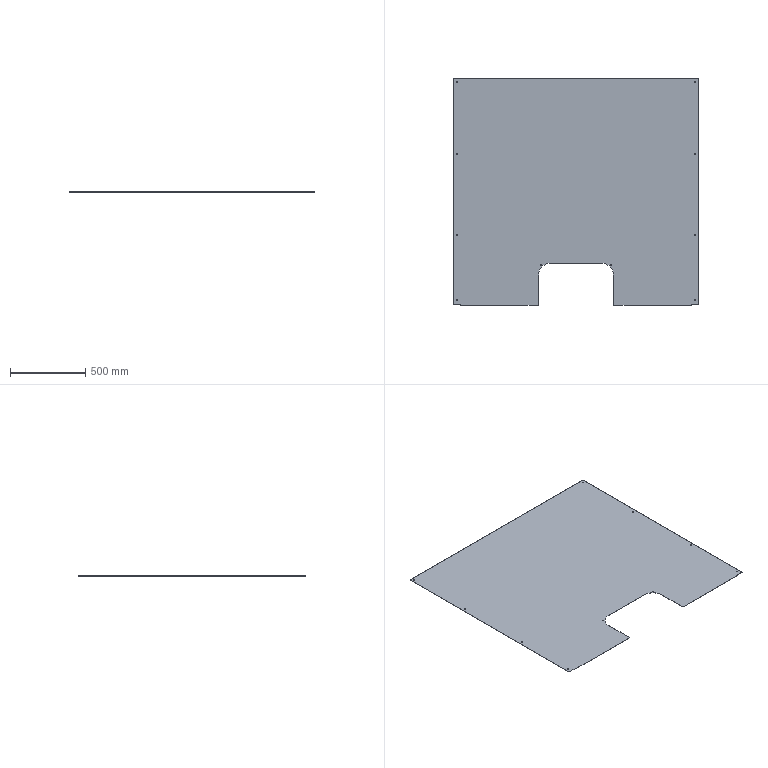Part | SolidWorks | features ICE 6, Fillet 3, HoleWzd 3, FlatPattern 1, SMBaseFlange 1, SheetMetal 1 | 1 solid | 44 faces | box 1628 x 1507 x 1.2 mm | volume 2778351 mm3 | cylinder 30 | plane 14 | commonest cylinder face diameters 7 x20 6 x8 160 x2
STEP:
#1=CARTESIAN_POINT('',(1511.5,-1240.,0.));
#2=VERTEX_POINT('',#1);
#3=CARTESIAN_POINT('',(1518.5,-1240.,0.));
#4=VERTEX_POINT('',#3);
#5=CARTESIAN_POINT('',(1515.,-1240.,0.));
#6=DIRECTION('',(0.,0.,1.));
#7=DIRECTION('',(1.,0.,0.));
#8=AXIS2_PLACEMENT_3D('',#5,#6,#7);
#9=CIRCLE('',#8,3.5);
#10=EDGE_CURVE('',#2,#4,#9,.T.);
#11=ORIENTED_EDGE('',*,*,#10,.F.);
#12=CARTESIAN_POINT('',(1511.5,-1240.,1.2));
#13=VERTEX_POINT('',#12);
#14=CARTESIAN_POINT('',(1511.5,-1240.,1.2));
#15=DIRECTION('',(0.,0.,1.));
#16=VECTOR('',#15,1000.);
#17=LINE('',#14,#16);
#18=EDGE_CURVE('',#2,#13,#17,.T.);
#19=ORIENTED_EDGE('',*,*,#18,.T.);
#20=CARTESIAN_POINT('',(1518.5,-1240.,1.2));
#21=VERTEX_POINT('',#20);
#22=CARTESIAN_POINT('',(1515.,-1240.,1.2));
#23=DIRECTION('',(0.,0.,1.));
#24=DIRECTION('',(1.,0.,0.));
#25=AXIS2_PLACEMENT_3D('',#22,#23,#24);
#26=CIRCLE('',#25,3.5);
#27=EDGE_CURVE('',#13,#21,#26,.T.);
#28=ORIENTED_EDGE('',*,*,#27,.T.);
#29=CARTESIAN_POINT('',(1518.5,-1240.,1.2));
#30=DIRECTION('',(0.,0.,1.));
#31=VECTOR('',#30,1000.);
#32=LINE('',#29,#31);
#33=EDGE_CURVE('',#4,#21,#32,.T.);
#34=ORIENTED_EDGE('',*,*,#33,.F.);
#35=EDGE_LOOP('',(#11,#19,#28,#34));
#36=FACE_OUTER_BOUND('',#35,.T.);
#37=CARTESIAN_POINT('',(1515.,-1240.,1.2));
#38=DIRECTION('',(0.,0.,1.));
#39=DIRECTION('',(1.,0.,0.));
#40=AXIS2_PLACEMENT_3D('',#37,#38,#39);
#41=CYLINDRICAL_SURFACE('',#40,3.5);
#42=ADVANCED_FACE('',(#36),#41,.F.);
#43=CARTESIAN_POINT('',(1981.5,-1240.,0.));
#44=VERTEX_POINT('',#43);
#45=CARTESIAN_POINT('',(1988.5,-1240.,0.));
#46=VERTEX_POINT('',#45);
#47=CARTESIAN_POINT('',(1985.,-1240.,0.));
#48=DIRECTION('',(0.,0.,1.));
#49=DIRECTION('',(1.,0.,0.));
#50=AXIS2_PLACEMENT_3D('',#47,#48,#49);
#51=CIRCLE('',#50,3.5);
#52=EDGE_CURVE('',#44,#46,#51,.T.);
#53=ORIENTED_EDGE('',*,*,#52,.F.);
#54=CARTESIAN_POINT('',(1981.5,-1240.,1.2));
#55=VERTEX_POINT('',#54);
#56=CARTESIAN_POINT('',(1981.5,-1240.,1.2));
#57=DIRECTION('',(0.,0.,1.));
#58=VECTOR('',#57,1000.);
#59=LINE('',#56,#58);
#60=EDGE_CURVE('',#44,#55,#59,.T.);
#61=ORIENTED_EDGE('',*,*,#60,.T.);
#62=CARTESIAN_POINT('',(1988.5,-1240.,1.2));
#63=VERTEX_POINT('',#62);
#64=CARTESIAN_POINT('',(1985.,-1240.,1.2));
#65=DIRECTION('',(0.,0.,1.));
#66=DIRECTION('',(1.,0.,0.));
#67=AXIS2_PLACEMENT_3D('',#64,#65,#66);
#68=CIRCLE('',#67,3.5);
#69=EDGE_CURVE('',#55,#63,#68,.T.);
#70=ORIENTED_EDGE('',*,*,#69,.T.);
#71=CARTESIAN_POINT('',(1988.5,-1240.,1.2));
#72=DIRECTION('',(0.,0.,1.));
#73=VECTOR('',#72,1000.);
#74=LINE('',#71,#73);
#75=EDGE_CURVE('',#46,#63,#74,.T.);
#76=ORIENTED_EDGE('',*,*,#75,.F.);
#77=EDGE_LOOP('',(#53,#61,#70,#76));
#78=FACE_OUTER_BOUND('',#77,.T.);
#79=CARTESIAN_POINT('',(1985.,-1240.,1.2));
#80=DIRECTION('',(0.,0.,1.));
#81=DIRECTION('',(1.,0.,0.));
#82=AXIS2_PLACEMENT_3D('',#79,#80,#81);
#83=CYLINDRICAL_SURFACE('',#82,3.5);
#84=ADVANCED_FACE('',(#78),#83,.F.);
#85=CARTESIAN_POINT('',(952.5,-20.,0.));
#86=VERTEX_POINT('',#85);
#87=CARTESIAN_POINT('',(959.5,-20.,0.));
#88=VERTEX_POINT('',#87);
#89=CARTESIAN_POINT('',(956.,-20.,0.));
#90=DIRECTION('',(0.,0.,1.));
#91=DIRECTION('',(1.,0.,0.));
#92=AXIS2_PLACEMENT_3D('',#89,#90,#91);
#93=CIRCLE('',#92,3.5);
#94=EDGE_CURVE('',#86,#88,#93,.T.);
#95=ORIENTED_EDGE('',*,*,#94,.F.);
#96=CARTESIAN_POINT('',(952.5,-20.,1.2));
#97=VERTEX_POINT('',#96);
#98=CARTESIAN_POINT('',(952.5,-20.,1.2));
#99=DIRECTION('',(0.,0.,1.));
#100=VECTOR('',#99,1000.);
#101=LINE('',#98,#100);
#102=EDGE_CURVE('',#86,#97,#101,.T.);
#103=ORIENTED_EDGE('',*,*,#102,.T.);
#104=CARTESIAN_POINT('',(959.5,-20.,1.2));
#105=VERTEX_POINT('',#104);
#106=CARTESIAN_POINT('',(956.,-20.,1.2));
#107=DIRECTION('',(0.,0.,1.));
#108=DIRECTION('',(1.,0.,0.));
#109=AXIS2_PLACEMENT_3D('',#106,#107,#108);
#110=CIRCLE('',#109,3.5);
#111=EDGE_CURVE('',#97,#105,#110,.T.);
#112=ORIENTED_EDGE('',*,*,#111,.T.);
#113=CARTESIAN_POINT('',(959.5,-20.,1.2));
#114=DIRECTION('',(0.,0.,1.));
#115=VECTOR('',#114,1000.);
#116=LINE('',#113,#115);
#117=EDGE_CURVE('',#88,#105,#116,.T.);
#118=ORIENTED_EDGE('',*,*,#117,.F.);
#119=EDGE_LOOP('',(#95,#103,#112,#118));
#120=FACE_OUTER_BOUND('',#119,.T.);
#121=CARTESIAN_POINT('',(956.,-20.,1.2));
#122=DIRECTION('',(0.,0.,1.));
#123=DIRECTION('',(1.,0.,0.));
#124=AXIS2_PLACEMENT_3D('',#121,#122,#123);
#125=CYLINDRICAL_SURFACE('',#124,3.5);
#126=ADVANCED_FACE('',(#120),#125,.F.);
#127=CARTESIAN_POINT('',(2540.5,-20.,0.));
#128=VERTEX_POINT('',#127);
#129=CARTESIAN_POINT('',(2547.5,-20.,0.));
#130=VERTEX_POINT('',#129);
#131=CARTESIAN_POINT('',(2544.,-20.,0.));
#132=DIRECTION('',(0.,0.,1.));
#133=DIRECTION('',(1.,0.,0.));
#134=AXIS2_PLACEMENT_3D('',#131,#132,#133);
#135=CIRCLE('',#134,3.5);
#136=EDGE_CURVE('',#128,#130,#135,.T.);
#137=ORIENTED_EDGE('',*,*,#136,.F.);
#138=CARTESIAN_POINT('',(2540.5,-20.,1.2));
#139=VERTEX_POINT('',#138);
#140=CARTESIAN_POINT('',(2540.5,-20.,1.2));
#141=DIRECTION('',(0.,0.,1.));
#142=VECTOR('',#141,1000.);
#143=LINE('',#140,#142);
#144=EDGE_CURVE('',#128,#139,#143,.T.);
#145=ORIENTED_EDGE('',*,*,#144,.T.);
#146=CARTESIAN_POINT('',(2547.5,-20.,1.2));
#147=VERTEX_POINT('',#146);
#148=CARTESIAN_POINT('',(2544.,-20.,1.2));
#149=DIRECTION('',(0.,0.,1.));
#150=DIRECTION('',(1.,0.,0.));
#151=AXIS2_PLACEMENT_3D('',#148,#149,#150);
#152=CIRCLE('',#151,3.5);
#153=EDGE_CURVE('',#139,#147,#152,.T.);
#154=ORIENTED_EDGE('',*,*,#153,.T.);
#155=CARTESIAN_POINT('',(2547.5,-20.,1.2));
#156=DIRECTION('',(0.,0.,1.));
#157=VECTOR('',#156,1000.);
#158=LINE('',#155,#157);
#159=EDGE_CURVE('',#130,#147,#158,.T.);
#160=ORIENTED_EDGE('',*,*,#159,.F.);
#161=EDGE_LOOP('',(#137,#145,#154,#160));
#162=FACE_OUTER_BOUND('',#161,.T.);
#163=CARTESIAN_POINT('',(2544.,-20.,1.2));
#164=DIRECTION('',(0.,0.,1.));
#165=DIRECTION('',(1.,0.,0.));
#166=AXIS2_PLACEMENT_3D('',#163,#164,#165);
#167=CYLINDRICAL_SURFACE('',#166,3.5);
#168=ADVANCED_FACE('',(#162),#167,.F.);
#169=CARTESIAN_POINT('',(952.5,-1471.,0.));
#170=VERTEX_POINT('',#169);
#171=CARTESIAN_POINT('',(959.5,-1471.,0.));
#172=VERTEX_POINT('',#171);
#173=CARTESIAN_POINT('',(956.,-1471.,0.));
#174=DIRECTION('',(0.,0.,1.));
#175=DIRECTION('',(1.,0.,0.));
#176=AXIS2_PLACEMENT_3D('',#173,#174,#175);
#177=CIRCLE('',#176,3.5);
#178=EDGE_CURVE('',#170,#172,#177,.T.);
#179=ORIENTED_EDGE('',*,*,#178,.F.);
#180=CARTESIAN_POINT('',(952.5,-1471.,1.2));
#181=VERTEX_POINT('',#180);
#182=CARTESIAN_POINT('',(952.5,-1471.,1.2));
#183=DIRECTION('',(0.,0.,1.));
#184=VECTOR('',#183,1000.);
#185=LINE('',#182,#184);
#186=EDGE_CURVE('',#170,#181,#185,.T.);
#187=ORIENTED_EDGE('',*,*,#186,.T.);
#188=CARTESIAN_POINT('',(959.5,-1471.,1.2));
#189=VERTEX_POINT('',#188);
#190=CARTESIAN_POINT('',(956.,-1471.,1.2));
#191=DIRECTION('',(0.,0.,1.));
#192=DIRECTION('',(1.,0.,0.));
#193=AXIS2_PLACEMENT_3D('',#190,#191,#192);
#194=CIRCLE('',#193,3.5);
#195=EDGE_CURVE('',#181,#189,#194,.T.);
#196=ORIENTED_EDGE('',*,*,#195,.T.);
#197=CARTESIAN_POINT('',(959.5,-1471.,1.2));
#198=DIRECTION('',(0.,0.,1.));
#199=VECTOR('',#198,1000.);
#200=LINE('',#197,#199);
#201=EDGE_CURVE('',#172,#189,#200,.T.);
#202=ORIENTED_EDGE('',*,*,#201,.F.);
#203=EDGE_LOOP('',(#179,#187,#196,#202));
#204=FACE_OUTER_BOUND('',#203,.T.);
#205=CARTESIAN_POINT('',(956.,-1471.,1.2));
#206=DIRECTION('',(0.,0.,1.));
#207=DIRECTION('',(1.,0.,0.));
#208=AXIS2_PLACEMENT_3D('',#205,#206,#207);
#209=CYLINDRICAL_SURFACE('',#208,3.5);
#210=ADVANCED_FACE('',(#204),#209,.F.);
#211=CARTESIAN_POINT('',(2540.5,-1471.,0.));
#212=VERTEX_POINT('',#211);
#213=CARTESIAN_POINT('',(2547.5,-1471.,0.));
#214=VERTEX_POINT('',#213);
#215=CARTESIAN_POINT('',(2544.,-1471.,0.));
#216=DIRECTION('',(0.,0.,1.));
#217=DIRECTION('',(1.,0.,0.));
#218=AXIS2_PLACEMENT_3D('',#215,#216,#217);
#219=CIRCLE('',#218,3.5);
#220=EDGE_CURVE('',#212,#214,#219,.T.);
#221=ORIENTED_EDGE('',*,*,#220,.F.);
#222=CARTESIAN_POINT('',(2540.5,-1471.,1.2));
#223=VERTEX_POINT('',#222);
#224=CARTESIAN_POINT('',(2540.5,-1471.,1.2));
#225=DIRECTION('',(0.,0.,1.));
#226=VECTOR('',#225,1000.);
#227=LINE('',#224,#226);
#228=EDGE_CURVE('',#212,#223,#227,.T.);
#229=ORIENTED_EDGE('',*,*,#228,.T.);
#230=CARTESIAN_POINT('',(2547.5,-1471.,1.2));
#231=VERTEX_POINT('',#230);
#232=CARTESIAN_POINT('',(2544.,-1471.,1.2));
#233=DIRECTION('',(0.,0.,1.));
#234=DIRECTION('',(1.,0.,0.));
#235=AXIS2_PLACEMENT_3D('',#232,#233,#234);
#236=CIRCLE('',#235,3.5);
#237=EDGE_CURVE('',#223,#231,#236,.T.);
#238=ORIENTED_EDGE('',*,*,#237,.T.);
#239=CARTESIAN_POINT('',(2547.5,-1471.,1.2));
#240=DIRECTION('',(0.,0.,1.));
#241=VECTOR('',#240,1000.);
#242=LINE('',#239,#241);
#243=EDGE_CURVE('',#214,#231,#242,.T.);
#244=ORIENTED_EDGE('',*,*,#243,.F.);
#245=EDGE_LOOP('',(#221,#229,#238,#244));
#246=FACE_OUTER_BOUND('',#245,.T.);
#247=CARTESIAN_POINT('',(2544.,-1471.,1.2));
#248=DIRECTION('',(0.,0.,1.));
#249=DIRECTION('',(1.,0.,0.));
#250=AXIS2_PLACEMENT_3D('',#247,#248,#249);
#251=CYLINDRICAL_SURFACE('',#250,3.5);
#252=ADVANCED_FACE('',(#246),#251,.F.);
#253=CARTESIAN_POINT('',(952.5,-1038.,0.));
#254=VERTEX_POINT('',#253);
#255=CARTESIAN_POINT('',(959.5,-1038.,0.));
#256=VERTEX_POINT('',#255);
#257=CARTESIAN_POINT('',(956.,-1038.,0.));
#258=DIRECTION('',(0.,0.,1.));
#259=DIRECTION('',(1.,0.,0.));
#260=AXIS2_PLACEMENT_3D('',#257,#258,#259);
#261=CIRCLE('',#260,3.5);
#262=EDGE_CURVE('',#254,#256,#261,.T.);
#263=ORIENTED_EDGE('',*,*,#262,.F.);
#264=CARTESIAN_POINT('',(952.5,-1038.,1.2));
#265=VERTEX_POINT('',#264);
#266=CARTESIAN_POINT('',(952.5,-1038.,1.2));
#267=DIRECTION('',(0.,0.,1.));
#268=VECTOR('',#267,1000.);
#269=LINE('',#266,#268);
#270=EDGE_CURVE('',#254,#265,#269,.T.);
#271=ORIENTED_EDGE('',*,*,#270,.T.);
#272=CARTESIAN_POINT('',(959.5,-1038.,1.2));
#273=VERTEX_POINT('',#272);
#274=CARTESIAN_POINT('',(956.,-1038.,1.2));
#275=DIRECTION('',(0.,0.,1.));
#276=DIRECTION('',(1.,0.,0.));
#277=AXIS2_PLACEMENT_3D('',#274,#275,#276);
#278=CIRCLE('',#277,3.5);
#279=EDGE_CURVE('',#265,#273,#278,.T.);
#280=ORIENTED_EDGE('',*,*,#279,.T.);
#281=CARTESIAN_POINT('',(959.5,-1038.,1.2));
#282=DIRECTION('',(0.,0.,1.));
#283=VECTOR('',#282,1000.);
#284=LINE('',#281,#283);
#285=EDGE_CURVE('',#256,#273,#284,.T.);
#286=ORIENTED_EDGE('',*,*,#285,.F.);
#287=EDGE_LOOP('',(#263,#271,#280,#286));
#288=FACE_OUTER_BOUND('',#287,.T.);
#289=CARTESIAN_POINT('',(956.,-1038.,1.2));
#290=DIRECTION('',(0.,0.,1.));
#291=DIRECTION('',(1.,0.,0.));
#292=AXIS2_PLACEMENT_3D('',#289,#290,#291);
#293=CYLINDRICAL_SURFACE('',#292,3.5);
#294=ADVANCED_FACE('',(#288),#293,.F.);
#295=CARTESIAN_POINT('',(2540.5,-1038.,0.));
#296=VERTEX_POINT('',#295);
#297=CARTESIAN_POINT('',(2547.5,-1038.,0.));
#298=VERTEX_POINT('',#297);
#299=CARTESIAN_POINT('',(2544.,-1038.,0.));
#300=DIRECTION('',(0.,0.,1.));
#301=DIRECTION('',(1.,0.,0.));
#302=AXIS2_PLACEMENT_3D('',#299,#300,#301);
#303=CIRCLE('',#302,3.5);
#304=EDGE_CURVE('',#296,#298,#303,.T.);
#305=ORIENTED_EDGE('',*,*,#304,.F.);
#306=CARTESIAN_POINT('',(2540.5,-1038.,1.2));
#307=VERTEX_POINT('',#306);
#308=CARTESIAN_POINT('',(2540.5,-1038.,1.2));
#309=DIRECTION('',(0.,0.,1.));
#310=VECTOR('',#309,1000.);
#311=LINE('',#308,#310);
#312=EDGE_CURVE('',#296,#307,#311,.T.);
#313=ORIENTED_EDGE('',*,*,#312,.T.);
#314=CARTESIAN_POINT('',(2547.5,-1038.,1.2));
#315=VERTEX_POINT('',#314);
#316=CARTESIAN_POINT('',(2544.,-1038.,1.2));
#317=DIRECTION('',(0.,0.,1.));
#318=DIRECTION('',(1.,0.,0.));
#319=AXIS2_PLACEMENT_3D('',#316,#317,#318);
#320=CIRCLE('',#319,3.5);
#321=EDGE_CURVE('',#307,#315,#320,.T.);
#322=ORIENTED_EDGE('',*,*,#321,.T.);
#323=CARTESIAN_POINT('',(2547.5,-1038.,1.2));
#324=DIRECTION('',(0.,0.,1.));
#325=VECTOR('',#324,1000.);
#326=LINE('',#323,#325);
#327=EDGE_CURVE('',#298,#315,#326,.T.);
#328=ORIENTED_EDGE('',*,*,#327,.F.);
#329=EDGE_LOOP('',(#305,#313,#322,#328));
#330=FACE_OUTER_BOUND('',#329,.T.);
#331=CARTESIAN_POINT('',(2544.,-1038.,1.2));
#332=DIRECTION('',(0.,0.,1.));
#333=DIRECTION('',(1.,0.,0.));
#334=AXIS2_PLACEMENT_3D('',#331,#332,#333);
#335=CYLINDRICAL_SURFACE('',#334,3.5);
#336=ADVANCED_FACE('',(#330),#335,.F.);
#337=CARTESIAN_POINT('',(952.5,-498.,0.));
#338=VERTEX_POINT('',#337);
#339=CARTESIAN_POINT('',(959.5,-498.,0.));
#340=VERTEX_POINT('',#339);
#341=CARTESIAN_POINT('',(956.,-498.,0.));
#342=DIRECTION('',(0.,0.,1.));
#343=DIRECTION('',(1.,0.,0.));
#344=AXIS2_PLACEMENT_3D('',#341,#342,#343);
#345=CIRCLE('',#344,3.5);
#346=EDGE_CURVE('',#338,#340,#345,.T.);
#347=ORIENTED_EDGE('',*,*,#346,.F.);
#348=CARTESIAN_POINT('',(952.5,-498.,1.2));
#349=VERTEX_POINT('',#348);
#350=CARTESIAN_POINT('',(952.5,-498.,1.2));
#351=DIRECTION('',(0.,0.,1.));
#352=VECTOR('',#351,1000.);
#353=LINE('',#350,#352);
#354=EDGE_CURVE('',#338,#349,#353,.T.);
#355=ORIENTED_EDGE('',*,*,#354,.T.);
#356=CARTESIAN_POINT('',(959.5,-498.,1.2));
#357=VERTEX_POINT('',#356);
#358=CARTESIAN_POINT('',(956.,-498.,1.2));
#359=DIRECTION('',(0.,0.,1.));
#360=DIRECTION('',(1.,0.,0.));
#361=AXIS2_PLACEMENT_3D('',#358,#359,#360);
#362=CIRCLE('',#361,3.5);
#363=EDGE_CURVE('',#349,#357,#362,.T.);
#364=ORIENTED_EDGE('',*,*,#363,.T.);
#365=CARTESIAN_POINT('',(959.5,-498.,1.2));
#366=DIRECTION('',(0.,0.,1.));
#367=VECTOR('',#366,1000.);
#368=LINE('',#365,#367);
#369=EDGE_CURVE('',#340,#357,#368,.T.);
#370=ORIENTED_EDGE('',*,*,#369,.F.);
#371=EDGE_LOOP('',(#347,#355,#364,#370));
#372=FACE_OUTER_BOUND('',#371,.T.);
#373=CARTESIAN_POINT('',(956.,-498.,1.2));
#374=DIRECTION('',(0.,0.,1.));
#375=DIRECTION('',(1.,0.,0.));
#376=AXIS2_PLACEMENT_3D('',#373,#374,#375);
#377=CYLINDRICAL_SURFACE('',#376,3.5);
#378=ADVANCED_FACE('',(#372),#377,.F.);
#379=CARTESIAN_POINT('',(2540.5,-498.,0.));
#380=VERTEX_POINT('',#379);
#381=CARTESIAN_POINT('',(2547.5,-498.,0.));
#382=VERTEX_POINT('',#381);
#383=CARTESIAN_POINT('',(2544.,-498.,0.));
#384=DIRECTION('',(0.,0.,1.));
#385=DIRECTION('',(1.,0.,0.));
#386=AXIS2_PLACEMENT_3D('',#383,#384,#385);
#387=CIRCLE('',#386,3.5);
#388=EDGE_CURVE('',#380,#382,#387,.T.);
#389=ORIENTED_EDGE('',*,*,#388,.F.);
#390=CARTESIAN_POINT('',(2540.5,-498.,1.2));
#391=VERTEX_POINT('',#390);
#392=CARTESIAN_POINT('',(2540.5,-498.,1.2));
#393=DIRECTION('',(0.,0.,1.));
#394=VECTOR('',#393,1000.);
#395=LINE('',#392,#394);
#396=EDGE_CURVE('',#380,#391,#395,.T.);
#397=ORIENTED_EDGE('',*,*,#396,.T.);
#398=CARTESIAN_POINT('',(2547.5,-498.,1.2));
#399=VERTEX_POINT('',#398);
#400=CARTESIAN_POINT('',(2544.,-498.,1.2));
#401=DIRECTION('',(0.,0.,1.));
#402=DIRECTION('',(1.,0.,0.));
#403=AXIS2_PLACEMENT_3D('',#400,#401,#402);
#404=CIRCLE('',#403,3.5);
#405=EDGE_CURVE('',#391,#399,#404,.T.);
#406=ORIENTED_EDGE('',*,*,#405,.T.);
#407=CARTESIAN_POINT('',(2547.5,-498.,1.2));
#408=DIRECTION('',(0.,0.,1.));
#409=VECTOR('',#408,1000.);
#410=LINE('',#407,#409);
#411=EDGE_CURVE('',#382,#399,#410,.T.);
#412=ORIENTED_EDGE('',*,*,#411,.F.);
#413=EDGE_LOOP('',(#389,#397,#406,#412));
#414=FACE_OUTER_BOUND('',#413,.T.);
#415=CARTESIAN_POINT('',(2544.,-498.,1.2));
#416=DIRECTION('',(0.,0.,1.));
#417=DIRECTION('',(1.,0.,0.));
#418=AXIS2_PLACEMENT_3D('',#415,#416,#417);
#419=CYLINDRICAL_SURFACE('',#418,3.5);
#420=ADVANCED_FACE('',(#414),#419,.F.);
#421=CARTESIAN_POINT('',(1497.,-1507.,1.2));
#422=VERTEX_POINT('',#421);
#423=CARTESIAN_POINT('',(984.,-1507.,1.2));
#424=VERTEX_POINT('',#423);
#425=CARTESIAN_POINT('',(890.,-1507.,1.2));
#426=DIRECTION('',(-1.,0.,0.));
#427=VECTOR('',#426,1000.);
#428=LINE('',#425,#427);
#429=EDGE_CURVE('',#422,#424,#428,.T.);
#430=ORIENTED_EDGE('',*,*,#429,.T.);
#431=CARTESIAN_POINT('',(984.,-1507.,0.));
#432=VERTEX_POINT('',#431);
#433=CARTESIAN_POINT('',(984.,-1507.,-8.8));
#434=DIRECTION('',(0.,0.,-1.));
#435=VECTOR('',#434,1000.);
#436=LINE('',#433,#435);
#437=EDGE_CURVE('',#424,#432,#436,.T.);
#438=ORIENTED_EDGE('',*,*,#437,.T.);
#439=CARTESIAN_POINT('',(1497.,-1507.,0.));
#440=VERTEX_POINT('',#439);
#441=CARTESIAN_POINT('',(0.,-1507.,0.));
#442=DIRECTION('',(-1.,0.,0.));
#443=VECTOR('',#442,1000.);
#444=LINE('',#441,#443);
#445=EDGE_CURVE('',#440,#432,#444,.T.);
#446=ORIENTED_EDGE('',*,*,#445,.F.);
#447=CARTESIAN_POINT('',(1497.,-1507.,-8.8));
#448=DIRECTION('',(0.,0.,1.));
#449=VECTOR('',#448,1000.);
#450=LINE('',#447,#449);
#451=EDGE_CURVE('',#440,#422,#450,.T.);
#452=ORIENTED_EDGE('',*,*,#451,.T.);
#453=EDGE_LOOP('',(#430,#438,#446,#452));
#454=FACE_OUTER_BOUND('',#453,.T.);
#455=CARTESIAN_POINT('',(890.,-1507.,-8.8));
#456=DIRECTION('',(0.,1.,0.));
#457=DIRECTION('',(0.,0.,1.));
#458=AXIS2_PLACEMENT_3D('',#455,#456,#457);
#459=PLANE('',#458);
#460=ADVANCED_FACE('',(#454),#459,.F.);
#461=CARTESIAN_POINT('',(939.,0.,0.));
#462=VERTEX_POINT('',#461);
#463=CARTESIAN_POINT('',(2561.,0.,0.));
#464=VERTEX_POINT('',#463);
#465=CARTESIAN_POINT('',(0.,0.,0.));
#466=DIRECTION('',(1.,0.,0.));
#467=VECTOR('',#466,1000.);
#468=LINE('',#465,#467);
#469=EDGE_CURVE('',#462,#464,#468,.T.);
#470=ORIENTED_EDGE('',*,*,#469,.F.);
#471=CARTESIAN_POINT('',(939.,0.,1.2));
#472=VERTEX_POINT('',#471);
#473=CARTESIAN_POINT('',(939.,0.,1.2));
#474=DIRECTION('',(0.,0.,1.));
#475=VECTOR('',#474,1000.);
#476=LINE('',#473,#475);
#477=EDGE_CURVE('',#462,#472,#476,.T.);
#478=ORIENTED_EDGE('',*,*,#477,.T.);
#479=CARTESIAN_POINT('',(2561.,0.,1.2));
#480=VERTEX_POINT('',#479);
#481=CARTESIAN_POINT('',(0.,0.,1.2));
#482=DIRECTION('',(1.,0.,0.));
#483=VECTOR('',#482,1000.);
#484=LINE('',#481,#483);
#485=EDGE_CURVE('',#472,#480,#484,.T.);
#486=ORIENTED_EDGE('',*,*,#485,.T.);
#487=CARTESIAN_POINT('',(2561.,0.,1.2));
#488=DIRECTION('',(0.,0.,-1.));
#489=VECTOR('',#488,1000.);
#490=LINE('',#487,#489);
#491=EDGE_CURVE('',#480,#464,#490,.T.);
#492=ORIENTED_EDGE('',*,*,#491,.T.);
#493=EDGE_LOOP('',(#470,#478,#486,#492));
#494=FACE_OUTER_BOUND('',#493,.T.);
#495=CARTESIAN_POINT('',(0.,0.,1.2));
#496=DIRECTION('',(0.,1.,0.));
#497=DIRECTION('',(0.,0.,1.));
#498=AXIS2_PLACEMENT_3D('',#495,#496,#497);
#499=PLANE('',#498);
#500=ADVANCED_FACE('',(#494),#499,.T.);
#501=CARTESIAN_POINT('',(1515.,-1240.,1.2));
#502=DIRECTION('',(0.,0.,1.));
#503=DIRECTION('',(1.,0.,0.));
#504=AXIS2_PLACEMENT_3D('',#501,#502,#503);
#505=CIRCLE('',#504,3.5);
#506=EDGE_CURVE('',#21,#13,#505,.T.);
#507=ORIENTED_EDGE('',*,*,#506,.F.);
#508=ORIENTED_EDGE('',*,*,#27,.F.);
#509=EDGE_LOOP('',(#507,#508));
#510=FACE_BOUND('',#509,.T.);
#511=CARTESIAN_POINT('',(1985.,-1240.,1.2));
#512=DIRECTION('',(0.,0.,1.));
#513=DIRECTION('',(1.,0.,0.));
#514=AXIS2_PLACEMENT_3D('',#511,#512,#513);
#515=CIRCLE('',#514,3.5);
#516=EDGE_CURVE('',#63,#55,#515,.T.);
#517=ORIENTED_EDGE('',*,*,#516,.F.);
#518=ORIENTED_EDGE('',*,*,#69,.F.);
#519=EDGE_LOOP('',(#517,#518));
#520=FACE_BOUND('',#519,.T.);
#521=CARTESIAN_POINT('',(956.,-20.,1.2));
#522=DIRECTION('',(0.,0.,1.));
#523=DIRECTION('',(1.,0.,0.));
#524=AXIS2_PLACEMENT_3D('',#521,#522,#523);
#525=CIRCLE('',#524,3.5);
#526=EDGE_CURVE('',#105,#97,#525,.T.);
#527=ORIENTED_EDGE('',*,*,#526,.F.);
#528=ORIENTED_EDGE('',*,*,#111,.F.);
#529=EDGE_LOOP('',(#527,#528));
#530=FACE_BOUND('',#529,.T.);
#531=CARTESIAN_POINT('',(2544.,-20.,1.2));
#532=DIRECTION('',(0.,0.,1.));
#533=DIRECTION('',(1.,0.,0.));
#534=AXIS2_PLACEMENT_3D('',#531,#532,#533);
#535=CIRCLE('',#534,3.5);
#536=EDGE_CURVE('',#147,#139,#535,.T.);
#537=ORIENTED_EDGE('',*,*,#536,.F.);
#538=ORIENTED_EDGE('',*,*,#153,.F.);
#539=EDGE_LOOP('',(#537,#538));
#540=FACE_BOUND('',#539,.T.);
#541=CARTESIAN_POINT('',(956.,-1471.,1.2));
#542=DIRECTION('',(0.,0.,1.));
#543=DIRECTION('',(1.,0.,0.));
#544=AXIS2_PLACEMENT_3D('',#541,#542,#543);
#545=CIRCLE('',#544,3.5);
#546=EDGE_CURVE('',#189,#181,#545,.T.);
#547=ORIENTED_EDGE('',*,*,#546,.F.);
#548=ORIENTED_EDGE('',*,*,#195,.F.);
#549=EDGE_LOOP('',(#547,#548));
#550=FACE_BOUND('',#549,.T.);
#551=CARTESIAN_POINT('',(2544.,-1471.,1.2));
#552=DIRECTION('',(0.,0.,1.));
#553=DIRECTION('',(1.,0.,0.));
#554=AXIS2_PLACEMENT_3D('',#551,#552,#553);
#555=CIRCLE('',#554,3.5);
#556=EDGE_CURVE('',#231,#223,#555,.T.);
#557=ORIENTED_EDGE('',*,*,#556,.F.);
#558=ORIENTED_EDGE('',*,*,#237,.F.);
#559=EDGE_LOOP('',(#557,#558));
#560=FACE_BOUND('',#559,.T.);
#561=CARTESIAN_POINT('',(956.,-1038.,1.2));
#562=DIRECTION('',(0.,0.,1.));
#563=DIRECTION('',(1.,0.,0.));
#564=AXIS2_PLACEMENT_3D('',#561,#562,#563);
#565=CIRCLE('',#564,3.5);
#566=EDGE_CURVE('',#273,#265,#565,.T.);
#567=ORIENTED_EDGE('',*,*,#566,.F.);
#568=ORIENTED_EDGE('',*,*,#279,.F.);
#569=EDGE_LOOP('',(#567,#568));
#570=FACE_BOUND('',#569,.T.);
#571=CARTESIAN_POINT('',(2544.,-1038.,1.2));
#572=DIRECTION('',(0.,0.,1.));
#573=DIRECTION('',(1.,0.,0.));
#574=AXIS2_PLACEMENT_3D('',#571,#572,#573);
#575=CIRCLE('',#574,3.5);
#576=EDGE_CURVE('',#315,#307,#575,.T.);
#577=ORIENTED_EDGE('',*,*,#576,.F.);
#578=ORIENTED_EDGE('',*,*,#321,.F.);
#579=EDGE_LOOP('',(#577,#578));
#580=FACE_BOUND('',#579,.T.);
#581=CARTESIAN_POINT('',(956.,-498.,1.2));
#582=DIRECTION('',(0.,0.,1.));
#583=DIRECTION('',(1.,0.,0.));
#584=AXIS2_PLACEMENT_3D('',#581,#582,#583);
#585=CIRCLE('',#584,3.5);
#586=EDGE_CURVE('',#357,#349,#585,.T.);
#587=ORIENTED_EDGE('',*,*,#586,.F.);
#588=ORIENTED_EDGE('',*,*,#363,.F.);
#589=EDGE_LOOP('',(#587,#588));
#590=FACE_BOUND('',#589,.T.);
#591=CARTESIAN_POINT('',(2544.,-498.,1.2));
#592=DIRECTION('',(0.,0.,1.));
#593=DIRECTION('',(1.,0.,0.));
#594=AXIS2_PLACEMENT_3D('',#591,#592,#593);
#595=CIRCLE('',#594,3.5);
#596=EDGE_CURVE('',#399,#391,#595,.T.);
#597=ORIENTED_EDGE('',*,*,#596,.F.);
#598=ORIENTED_EDGE('',*,*,#405,.F.);
#599=EDGE_LOOP('',(#597,#598));
#600=FACE_BOUND('',#599,.T.);
#601=ORIENTED_EDGE('',*,*,#485,.F.);
#602=CARTESIAN_POINT('',(936.,-3.,1.2));
#603=VERTEX_POINT('',#602);
#604=CARTESIAN_POINT('',(939.,-3.,1.2));
#605=DIRECTION('',(0.,0.,1.));
#606=DIRECTION('',(1.,0.,0.));
#607=AXIS2_PLACEMENT_3D('',#604,#605,#606);
#608=CIRCLE('',#607,3.);
#609=EDGE_CURVE('',#472,#603,#608,.T.);
#610=ORIENTED_EDGE('',*,*,#609,.T.);
#611=CARTESIAN_POINT('',(936.,-1499.,1.2));
#612=VERTEX_POINT('',#611);
#613=CARTESIAN_POINT('',(936.,-1651.39,1.2));
#614=DIRECTION('',(0.,-1.,0.));
#615=VECTOR('',#614,1000.);
#616=LINE('',#613,#615);
#617=EDGE_CURVE('',#603,#612,#616,.T.);
#618=ORIENTED_EDGE('',*,*,#617,.T.);
#619=CARTESIAN_POINT('',(939.,-1502.,1.2));
#620=VERTEX_POINT('',#619);
#621=CARTESIAN_POINT('',(939.,-1499.,1.2));
#622=DIRECTION('',(0.,0.,1.));
#623=DIRECTION('',(1.,0.,0.));
#624=AXIS2_PLACEMENT_3D('',#621,#622,#623);
#625=CIRCLE('',#624,3.);
#626=EDGE_CURVE('',#612,#620,#625,.T.);
#627=ORIENTED_EDGE('',*,*,#626,.T.);
#628=CARTESIAN_POINT('',(981.,-1502.,1.2));
#629=VERTEX_POINT('',#628);
#630=CARTESIAN_POINT('',(936.,-1502.,1.2));
#631=DIRECTION('',(-1.,0.,0.));
#632=VECTOR('',#631,1000.);
#633=LINE('',#630,#632);
#634=EDGE_CURVE('',#629,#620,#633,.T.);
#635=ORIENTED_EDGE('',*,*,#634,.F.);
#636=CARTESIAN_POINT('',(981.,-1504.,1.2));
#637=VERTEX_POINT('',#636);
#638=CARTESIAN_POINT('',(981.,-1507.,1.2));
#639=DIRECTION('',(0.,1.,0.));
#640=VECTOR('',#639,1000.);
#641=LINE('',#638,#640);
#642=EDGE_CURVE('',#637,#629,#641,.T.);
#643=ORIENTED_EDGE('',*,*,#642,.F.);
#644=CARTESIAN_POINT('',(984.,-1504.,1.2));
#645=DIRECTION('',(0.,0.,1.));
#646=DIRECTION('',(1.,0.,0.));
#647=AXIS2_PLACEMENT_3D('',#644,#645,#646);
#648=CIRCLE('',#647,3.);
#649=EDGE_CURVE('',#637,#424,#648,.T.);
#650=ORIENTED_EDGE('',*,*,#649,.T.);
#651=ORIENTED_EDGE('',*,*,#429,.F.);
#652=CARTESIAN_POINT('',(1500.,-1504.,1.2));
#653=VERTEX_POINT('',#652);
#654=CARTESIAN_POINT('',(1497.,-1504.,1.2));
#655=DIRECTION('',(0.,0.,1.));
#656=DIRECTION('',(1.,0.,0.));
#657=AXIS2_PLACEMENT_3D('',#654,#655,#656);
#658=CIRCLE('',#657,3.);
#659=EDGE_CURVE('',#422,#653,#658,.T.);
#660=ORIENTED_EDGE('',*,*,#659,.T.);
#661=CARTESIAN_POINT('',(1500.,-1307.,1.2));
#662=VERTEX_POINT('',#661);
#663=CARTESIAN_POINT('',(1500.,-1507.,1.2));
#664=DIRECTION('',(0.,-1.,0.));
#665=VECTOR('',#664,1000.);
#666=LINE('',#663,#665);
#667=EDGE_CURVE('',#662,#653,#666,.T.);
#668=ORIENTED_EDGE('',*,*,#667,.F.);
#669=CARTESIAN_POINT('',(1580.,-1227.,1.2));
#670=VERTEX_POINT('',#669);
#671=CARTESIAN_POINT('',(1580.,-1307.,1.2));
#672=DIRECTION('',(0.,0.,-1.));
#673=DIRECTION('',(1.,0.,0.));
#674=AXIS2_PLACEMENT_3D('',#671,#672,#673);
#675=CIRCLE('',#674,80.);
#676=EDGE_CURVE('',#662,#670,#675,.T.);
#677=ORIENTED_EDGE('',*,*,#676,.T.);
#678=CARTESIAN_POINT('',(1920.,-1227.,1.2));
#679=VERTEX_POINT('',#678);
#680=CARTESIAN_POINT('',(1500.,-1227.,1.2));
#681=DIRECTION('',(-1.,0.,0.));
#682=VECTOR('',#681,1000.);
#683=LINE('',#680,#682);
#684=EDGE_CURVE('',#679,#670,#683,.T.);
#685=ORIENTED_EDGE('',*,*,#684,.F.);
#686=CARTESIAN_POINT('',(2000.,-1307.,1.2));
#687=VERTEX_POINT('',#686);
#688=CARTESIAN_POINT('',(1920.,-1307.,1.2));
#689=DIRECTION('',(0.,0.,-1.));
#690=DIRECTION('',(1.,0.,0.));
#691=AXIS2_PLACEMENT_3D('',#688,#689,#690);
#692=CIRCLE('',#691,80.);
#693=EDGE_CURVE('',#679,#687,#692,.T.);
#694=ORIENTED_EDGE('',*,*,#693,.T.);
#695=CARTESIAN_POINT('',(2000.,-1504.,1.2));
#696=VERTEX_POINT('',#695);
#697=CARTESIAN_POINT('',(2000.,-1227.,1.2));
#698=DIRECTION('',(0.,1.,0.));
#699=VECTOR('',#698,1000.);
#700=LINE('',#697,#699);
#701=EDGE_CURVE('',#696,#687,#700,.T.);
#702=ORIENTED_EDGE('',*,*,#701,.F.);
#703=CARTESIAN_POINT('',(2003.,-1507.,1.2));
#704=VERTEX_POINT('',#703);
#705=CARTESIAN_POINT('',(2003.,-1504.,1.2));
#706=DIRECTION('',(0.,0.,1.));
#707=DIRECTION('',(1.,0.,0.));
#708=AXIS2_PLACEMENT_3D('',#705,#706,#707);
#709=CIRCLE('',#708,3.);
#710=EDGE_CURVE('',#696,#704,#709,.T.);
#711=ORIENTED_EDGE('',*,*,#710,.T.);
#712=CARTESIAN_POINT('',(2516.,-1507.,1.2));
#713=VERTEX_POINT('',#712);
#714=CARTESIAN_POINT('',(890.,-1507.,1.2));
#715=DIRECTION('',(-1.,0.,0.));
#716=VECTOR('',#715,1000.);
#717=LINE('',#714,#716);
#718=EDGE_CURVE('',#713,#704,#717,.T.);
#719=ORIENTED_EDGE('',*,*,#718,.F.);
#720=CARTESIAN_POINT('',(2519.,-1504.,1.2));
#721=VERTEX_POINT('',#720);
#722=CARTESIAN_POINT('',(2516.,-1504.,1.2));
#723=DIRECTION('',(0.,0.,1.));
#724=DIRECTION('',(1.,0.,0.));
#725=AXIS2_PLACEMENT_3D('',#722,#723,#724);
#726=CIRCLE('',#725,3.);
#727=EDGE_CURVE('',#713,#721,#726,.T.);
#728=ORIENTED_EDGE('',*,*,#727,.T.);
#729=CARTESIAN_POINT('',(2519.,-1502.,1.2));
#730=VERTEX_POINT('',#729);
#731=CARTESIAN_POINT('',(2519.,-1507.,1.2));
#732=DIRECTION('',(0.,-1.,0.));
#733=VECTOR('',#732,1000.);
#734=LINE('',#731,#733);
#735=EDGE_CURVE('',#730,#721,#734,.T.);
#736=ORIENTED_EDGE('',*,*,#735,.F.);
#737=CARTESIAN_POINT('',(2561.,-1502.,1.2));
#738=VERTEX_POINT('',#737);
#739=CARTESIAN_POINT('',(2564.,-1502.,1.2));
#740=DIRECTION('',(-1.,0.,0.));
#741=VECTOR('',#740,1000.);
#742=LINE('',#739,#741);
#743=EDGE_CURVE('',#738,#730,#742,.T.);
#744=ORIENTED_EDGE('',*,*,#743,.F.);
#745=CARTESIAN_POINT('',(2564.,-1499.,1.2));
#746=VERTEX_POINT('',#745);
#747=CARTESIAN_POINT('',(2561.,-1499.,1.2));
#748=DIRECTION('',(0.,0.,1.));
#749=DIRECTION('',(1.,0.,0.));
#750=AXIS2_PLACEMENT_3D('',#747,#748,#749);
#751=CIRCLE('',#750,3.);
#752=EDGE_CURVE('',#738,#746,#751,.T.);
#753=ORIENTED_EDGE('',*,*,#752,.T.);
#754=CARTESIAN_POINT('',(2564.,-3.,1.2));
#755=VERTEX_POINT('',#754);
#756=CARTESIAN_POINT('',(2564.,-1651.39,1.2));
#757=DIRECTION('',(0.,1.,0.));
#758=VECTOR('',#757,1000.);
#759=LINE('',#756,#758);
#760=EDGE_CURVE('',#746,#755,#759,.T.);
#761=ORIENTED_EDGE('',*,*,#760,.T.);
#762=CARTESIAN_POINT('',(2561.,-3.,1.2));
#763=DIRECTION('',(0.,0.,1.));
#764=DIRECTION('',(1.,0.,0.));
#765=AXIS2_PLACEMENT_3D('',#762,#763,#764);
#766=CIRCLE('',#765,3.);
#767=EDGE_CURVE('',#755,#480,#766,.T.);
#768=ORIENTED_EDGE('',*,*,#767,.T.);
#769=EDGE_LOOP('',(#601,#610,#618,#627,#635,#643,#650,#651,#660,#668,#677,#685,#694,#702,#711,#719,#728,#736,#744,#753,#761,#768));
#770=FACE_OUTER_BOUND('',#769,.T.);
#771=CARTESIAN_POINT('',(0.,0.,1.2));
#772=DIRECTION('',(0.,0.,1.));
#773=DIRECTION('',(1.,0.,0.));
#774=AXIS2_PLACEMENT_3D('',#771,#772,#773);
#775=PLANE('',#774);
#776=ADVANCED_FACE('',(#510,#520,#530,#540,#550,#560,#570,#580,#590,#600,#770),#775,.T.);
#777=CARTESIAN_POINT('',(1515.,-1240.,0.));
#778=DIRECTION('',(0.,0.,1.));
#779=DIRECTION('',(1.,0.,0.));
#780=AXIS2_PLACEMENT_3D('',#777,#778,#779);
#781=CIRCLE('',#780,3.5);
#782=EDGE_CURVE('',#4,#2,#781,.T.);
#783=ORIENTED_EDGE('',*,*,#782,.T.);
#784=ORIENTED_EDGE('',*,*,#10,.T.);
#785=EDGE_LOOP('',(#783,#784));
#786=FACE_BOUND('',#785,.T.);
#787=CARTESIAN_POINT('',(1985.,-1240.,0.));
#788=DIRECTION('',(0.,0.,1.));
#789=DIRECTION('',(1.,0.,0.));
#790=AXIS2_PLACEMENT_3D('',#787,#788,#789);
#791=CIRCLE('',#790,3.5);
#792=EDGE_CURVE('',#46,#44,#791,.T.);
#793=ORIENTED_EDGE('',*,*,#792,.T.);
#794=ORIENTED_EDGE('',*,*,#52,.T.);
#795=EDGE_LOOP('',(#793,#794));
#796=FACE_BOUND('',#795,.T.);
#797=CARTESIAN_POINT('',(956.,-20.,0.));
#798=DIRECTION('',(0.,0.,1.));
#799=DIRECTION('',(1.,0.,0.));
#800=AXIS2_PLACEMENT_3D('',#797,#798,#799);
#801=CIRCLE('',#800,3.5);
#802=EDGE_CURVE('',#88,#86,#801,.T.);
#803=ORIENTED_EDGE('',*,*,#802,.T.);
#804=ORIENTED_EDGE('',*,*,#94,.T.);
#805=EDGE_LOOP('',(#803,#804));
#806=FACE_BOUND('',#805,.T.);
#807=CARTESIAN_POINT('',(2544.,-20.,0.));
#808=DIRECTION('',(0.,0.,1.));
#809=DIRECTION('',(1.,0.,0.));
#810=AXIS2_PLACEMENT_3D('',#807,#808,#809);
#811=CIRCLE('',#810,3.5);
#812=EDGE_CURVE('',#130,#128,#811,.T.);
#813=ORIENTED_EDGE('',*,*,#812,.T.);
#814=ORIENTED_EDGE('',*,*,#136,.T.);
#815=EDGE_LOOP('',(#813,#814));
#816=FACE_BOUND('',#815,.T.);
#817=CARTESIAN_POINT('',(956.,-1471.,0.));
#818=DIRECTION('',(0.,0.,1.));
#819=DIRECTION('',(1.,0.,0.));
#820=AXIS2_PLACEMENT_3D('',#817,#818,#819);
#821=CIRCLE('',#820,3.5);
#822=EDGE_CURVE('',#172,#170,#821,.T.);
#823=ORIENTED_EDGE('',*,*,#822,.T.);
#824=ORIENTED_EDGE('',*,*,#178,.T.);
#825=EDGE_LOOP('',(#823,#824));
#826=FACE_BOUND('',#825,.T.);
#827=CARTESIAN_POINT('',(2544.,-1471.,0.));
#828=DIRECTION('',(0.,0.,1.));
#829=DIRECTION('',(1.,0.,0.));
#830=AXIS2_PLACEMENT_3D('',#827,#828,#829);
#831=CIRCLE('',#830,3.5);
#832=EDGE_CURVE('',#214,#212,#831,.T.);
#833=ORIENTED_EDGE('',*,*,#832,.T.);
#834=ORIENTED_EDGE('',*,*,#220,.T.);
#835=EDGE_LOOP('',(#833,#834));
#836=FACE_BOUND('',#835,.T.);
#837=CARTESIAN_POINT('',(956.,-1038.,0.));
#838=DIRECTION('',(0.,0.,1.));
#839=DIRECTION('',(1.,0.,0.));
#840=AXIS2_PLACEMENT_3D('',#837,#838,#839);
#841=CIRCLE('',#840,3.5);
#842=EDGE_CURVE('',#256,#254,#841,.T.);
#843=ORIENTED_EDGE('',*,*,#842,.T.);
#844=ORIENTED_EDGE('',*,*,#262,.T.);
#845=EDGE_LOOP('',(#843,#844));
#846=FACE_BOUND('',#845,.T.);
#847=CARTESIAN_POINT('',(2544.,-1038.,0.));
#848=DIRECTION('',(0.,0.,1.));
#849=DIRECTION('',(1.,0.,0.));
#850=AXIS2_PLACEMENT_3D('',#847,#848,#849);
#851=CIRCLE('',#850,3.5);
#852=EDGE_CURVE('',#298,#296,#851,.T.);
#853=ORIENTED_EDGE('',*,*,#852,.T.);
#854=ORIENTED_EDGE('',*,*,#304,.T.);
#855=EDGE_LOOP('',(#853,#854));
#856=FACE_BOUND('',#855,.T.);
#857=CARTESIAN_POINT('',(956.,-498.,0.));
#858=DIRECTION('',(0.,0.,1.));
#859=DIRECTION('',(1.,0.,0.));
#860=AXIS2_PLACEMENT_3D('',#857,#858,#859);
#861=CIRCLE('',#860,3.5);
#862=EDGE_CURVE('',#340,#338,#861,.T.);
#863=ORIENTED_EDGE('',*,*,#862,.T.);
#864=ORIENTED_EDGE('',*,*,#346,.T.);
#865=EDGE_LOOP('',(#863,#864));
#866=FACE_BOUND('',#865,.T.);
#867=CARTESIAN_POINT('',(2544.,-498.,0.));
#868=DIRECTION('',(0.,0.,1.));
#869=DIRECTION('',(1.,0.,0.));
#870=AXIS2_PLACEMENT_3D('',#867,#868,#869);
#871=CIRCLE('',#870,3.5);
#872=EDGE_CURVE('',#382,#380,#871,.T.);
#873=ORIENTED_EDGE('',*,*,#872,.T.);
#874=ORIENTED_EDGE('',*,*,#388,.T.);
#875=EDGE_LOOP('',(#873,#874));
#876=FACE_BOUND('',#875,.T.);
#877=CARTESIAN_POINT('',(936.,-3.,0.));
#878=VERTEX_POINT('',#877);
#879=CARTESIAN_POINT('',(936.,-1499.,0.));
#880=VERTEX_POINT('',#879);
#881=CARTESIAN_POINT('',(936.,0.,0.));
#882=DIRECTION('',(0.,-1.,0.));
#883=VECTOR('',#882,1000.);
#884=LINE('',#881,#883);
#885=EDGE_CURVE('',#878,#880,#884,.T.);
#886=ORIENTED_EDGE('',*,*,#885,.F.);
#887=CARTESIAN_POINT('',(939.,-3.,0.));
#888=DIRECTION('',(0.,0.,-1.));
#889=DIRECTION('',(1.,0.,0.));
#890=AXIS2_PLACEMENT_3D('',#887,#888,#889);
#891=CIRCLE('',#890,3.);
#892=EDGE_CURVE('',#878,#462,#891,.T.);
#893=ORIENTED_EDGE('',*,*,#892,.T.);
#894=ORIENTED_EDGE('',*,*,#469,.T.);
#895=CARTESIAN_POINT('',(2564.,-3.,0.));
#896=VERTEX_POINT('',#895);
#897=CARTESIAN_POINT('',(2561.,-3.,0.));
#898=DIRECTION('',(0.,0.,-1.));
#899=DIRECTION('',(1.,0.,0.));
#900=AXIS2_PLACEMENT_3D('',#897,#898,#899);
#901=CIRCLE('',#900,3.);
#902=EDGE_CURVE('',#464,#896,#901,.T.);
#903=ORIENTED_EDGE('',*,*,#902,.T.);
#904=CARTESIAN_POINT('',(2564.,-1499.,0.));
#905=VERTEX_POINT('',#904);
#906=CARTESIAN_POINT('',(2564.,0.,0.));
#907=DIRECTION('',(0.,1.,0.));
#908=VECTOR('',#907,1000.);
#909=LINE('',#906,#908);
#910=EDGE_CURVE('',#905,#896,#909,.T.);
#911=ORIENTED_EDGE('',*,*,#910,.F.);
#912=CARTESIAN_POINT('',(2561.,-1502.,0.));
#913=VERTEX_POINT('',#912);
#914=CARTESIAN_POINT('',(2561.,-1499.,0.));
#915=DIRECTION('',(0.,0.,-1.));
#916=DIRECTION('',(1.,0.,0.));
#917=AXIS2_PLACEMENT_3D('',#914,#915,#916);
#918=CIRCLE('',#917,3.);
#919=EDGE_CURVE('',#905,#913,#918,.T.);
#920=ORIENTED_EDGE('',*,*,#919,.T.);
#921=CARTESIAN_POINT('',(2519.,-1502.,0.));
#922=VERTEX_POINT('',#921);
#923=CARTESIAN_POINT('',(0.,-1502.,0.));
#924=DIRECTION('',(-1.,0.,0.));
#925=VECTOR('',#924,1000.);
#926=LINE('',#923,#925);
#927=EDGE_CURVE('',#913,#922,#926,.T.);
#928=ORIENTED_EDGE('',*,*,#927,.T.);
#929=CARTESIAN_POINT('',(2519.,-1504.,0.));
#930=VERTEX_POINT('',#929);
#931=CARTESIAN_POINT('',(2519.,0.,0.));
#932=DIRECTION('',(0.,-1.,0.));
#933=VECTOR('',#932,1000.);
#934=LINE('',#931,#933);
#935=EDGE_CURVE('',#922,#930,#934,.T.);
#936=ORIENTED_EDGE('',*,*,#935,.T.);
#937=CARTESIAN_POINT('',(2516.,-1507.,0.));
#938=VERTEX_POINT('',#937);
#939=CARTESIAN_POINT('',(2516.,-1504.,0.));
#940=DIRECTION('',(0.,0.,-1.));
#941=DIRECTION('',(1.,0.,0.));
#942=AXIS2_PLACEMENT_3D('',#939,#940,#941);
#943=CIRCLE('',#942,3.);
#944=EDGE_CURVE('',#930,#938,#943,.T.);
#945=ORIENTED_EDGE('',*,*,#944,.T.);
#946=CARTESIAN_POINT('',(2003.,-1507.,0.));
#947=VERTEX_POINT('',#946);
#948=CARTESIAN_POINT('',(0.,-1507.,0.));
#949=DIRECTION('',(-1.,0.,0.));
#950=VECTOR('',#949,1000.);
#951=LINE('',#948,#950);
#952=EDGE_CURVE('',#938,#947,#951,.T.);
#953=ORIENTED_EDGE('',*,*,#952,.T.);
#954=CARTESIAN_POINT('',(2000.,-1504.,0.));
#955=VERTEX_POINT('',#954);
#956=CARTESIAN_POINT('',(2003.,-1504.,0.));
#957=DIRECTION('',(0.,0.,-1.));
#958=DIRECTION('',(1.,0.,0.));
#959=AXIS2_PLACEMENT_3D('',#956,#957,#958);
#960=CIRCLE('',#959,3.);
#961=EDGE_CURVE('',#947,#955,#960,.T.);
#962=ORIENTED_EDGE('',*,*,#961,.T.);
#963=CARTESIAN_POINT('',(2000.,-1307.,0.));
#964=VERTEX_POINT('',#963);
#965=CARTESIAN_POINT('',(2000.,0.,0.));
#966=DIRECTION('',(0.,1.,0.));
#967=VECTOR('',#966,1000.);
#968=LINE('',#965,#967);
#969=EDGE_CURVE('',#955,#964,#968,.T.);
#970=ORIENTED_EDGE('',*,*,#969,.T.);
#971=CARTESIAN_POINT('',(1920.,-1227.,0.));
#972=VERTEX_POINT('',#971);
#973=CARTESIAN_POINT('',(1920.,-1307.,0.));
#974=DIRECTION('',(0.,0.,1.));
#975=DIRECTION('',(1.,0.,0.));
#976=AXIS2_PLACEMENT_3D('',#973,#974,#975);
#977=CIRCLE('',#976,80.);
#978=EDGE_CURVE('',#964,#972,#977,.T.);
#979=ORIENTED_EDGE('',*,*,#978,.T.);
#980=CARTESIAN_POINT('',(1580.,-1227.,0.));
#981=VERTEX_POINT('',#980);
#982=CARTESIAN_POINT('',(0.,-1227.,0.));
#983=DIRECTION('',(-1.,0.,0.));
#984=VECTOR('',#983,1000.);
#985=LINE('',#982,#984);
#986=EDGE_CURVE('',#972,#981,#985,.T.);
#987=ORIENTED_EDGE('',*,*,#986,.T.);
#988=CARTESIAN_POINT('',(1500.,-1307.,0.));
#989=VERTEX_POINT('',#988);
#990=CARTESIAN_POINT('',(1580.,-1307.,0.));
#991=DIRECTION('',(0.,0.,1.));
#992=DIRECTION('',(1.,0.,0.));
#993=AXIS2_PLACEMENT_3D('',#990,#991,#992);
#994=CIRCLE('',#993,80.);
#995=EDGE_CURVE('',#981,#989,#994,.T.);
#996=ORIENTED_EDGE('',*,*,#995,.T.);
#997=CARTESIAN_POINT('',(1500.,-1504.,0.));
#998=VERTEX_POINT('',#997);
#999=CARTESIAN_POINT('',(1500.,0.,0.));
#1000=DIRECTION('',(0.,-1.,0.));
#1001=VECTOR('',#1000,1000.);
#1002=LINE('',#999,#1001);
#1003=EDGE_CURVE('',#989,#998,#1002,.T.);
#1004=ORIENTED_EDGE('',*,*,#1003,.T.);
#1005=CARTESIAN_POINT('',(1497.,-1504.,0.));
#1006=DIRECTION('',(0.,0.,-1.));
#1007=DIRECTION('',(1.,0.,0.));
#1008=AXIS2_PLACEMENT_3D('',#1005,#1006,#1007);
#1009=CIRCLE('',#1008,3.);
#1010=EDGE_CURVE('',#998,#440,#1009,.T.);
#1011=ORIENTED_EDGE('',*,*,#1010,.T.);
#1012=ORIENTED_EDGE('',*,*,#445,.T.);
#1013=CARTESIAN_POINT('',(981.,-1504.,0.));
#1014=VERTEX_POINT('',#1013);
#1015=CARTESIAN_POINT('',(984.,-1504.,0.));
#1016=DIRECTION('',(0.,0.,-1.));
#1017=DIRECTION('',(1.,0.,0.));
#1018=AXIS2_PLACEMENT_3D('',#1015,#1016,#1017);
#1019=CIRCLE('',#1018,3.);
#1020=EDGE_CURVE('',#432,#1014,#1019,.T.);
#1021=ORIENTED_EDGE('',*,*,#1020,.T.);
#1022=CARTESIAN_POINT('',(981.,-1502.,0.));
#1023=VERTEX_POINT('',#1022);
#1024=CARTESIAN_POINT('',(981.,0.,0.));
#1025=DIRECTION('',(0.,1.,0.));
#1026=VECTOR('',#1025,1000.);
#1027=LINE('',#1024,#1026);
#1028=EDGE_CURVE('',#1014,#1023,#1027,.T.);
#1029=ORIENTED_EDGE('',*,*,#1028,.T.);
#1030=CARTESIAN_POINT('',(939.,-1502.,0.));
#1031=VERTEX_POINT('',#1030);
#1032=CARTESIAN_POINT('',(0.,-1502.,0.));
#1033=DIRECTION('',(-1.,0.,0.));
#1034=VECTOR('',#1033,1000.);
#1035=LINE('',#1032,#1034);
#1036=EDGE_CURVE('',#1023,#1031,#1035,.T.);
#1037=ORIENTED_EDGE('',*,*,#1036,.T.);
#1038=CARTESIAN_POINT('',(939.,-1499.,0.));
#1039=DIRECTION('',(0.,0.,-1.));
#1040=DIRECTION('',(1.,0.,0.));
#1041=AXIS2_PLACEMENT_3D('',#1038,#1039,#1040);
#1042=CIRCLE('',#1041,3.);
#1043=EDGE_CURVE('',#1031,#880,#1042,.T.);
#1044=ORIENTED_EDGE('',*,*,#1043,.T.);
#1045=EDGE_LOOP('',(#886,#893,#894,#903,#911,#920,#928,#936,#945,#953,#962,#970,#979,#987,#996,#1004,#1011,#1012,#1021,#1029,#1037,#1044));
#1046=FACE_OUTER_BOUND('',#1045,.T.);
#1047=CARTESIAN_POINT('',(0.,0.,0.));
#1048=DIRECTION('',(0.,0.,1.));
#1049=DIRECTION('',(1.,0.,0.));
#1050=AXIS2_PLACEMENT_3D('',#1047,#1048,#1049);
#1051=PLANE('',#1050);
#1052=ADVANCED_FACE('',(#786,#796,#806,#816,#826,#836,#846,#856,#866,#876,#1046),#1051,.F.);
#1053=ORIENTED_EDGE('',*,*,#718,.T.);
#1054=CARTESIAN_POINT('',(2003.,-1507.,-8.8));
#1055=DIRECTION('',(0.,0.,-1.));
#1056=VECTOR('',#1055,1000.);
#1057=LINE('',#1054,#1056);
#1058=EDGE_CURVE('',#704,#947,#1057,.T.);
#1059=ORIENTED_EDGE('',*,*,#1058,.T.);
#1060=ORIENTED_EDGE('',*,*,#952,.F.);
#1061=CARTESIAN_POINT('',(2516.,-1507.,-8.8));
#1062=DIRECTION('',(0.,0.,1.));
#1063=VECTOR('',#1062,1000.);
#1064=LINE('',#1061,#1063);
#1065=EDGE_CURVE('',#938,#713,#1064,.T.);
#1066=ORIENTED_EDGE('',*,*,#1065,.T.);
#1067=EDGE_LOOP('',(#1053,#1059,#1060,#1066));
#1068=FACE_OUTER_BOUND('',#1067,.T.);
#1069=CARTESIAN_POINT('',(890.,-1507.,-8.8));
#1070=DIRECTION('',(0.,1.,0.));
#1071=DIRECTION('',(0.,0.,1.));
#1072=AXIS2_PLACEMENT_3D('',#1069,#1070,#1071);
#1073=PLANE('',#1072);
#1074=ADVANCED_FACE('',(#1068),#1073,.F.);
#1075=ORIENTED_EDGE('',*,*,#986,.F.);
#1076=CARTESIAN_POINT('',(1920.,-1227.,1.2));
#1077=DIRECTION('',(0.,0.,1.));
#1078=VECTOR('',#1077,1000.);
#1079=LINE('',#1076,#1078);
#1080=EDGE_CURVE('',#972,#679,#1079,.T.);
#1081=ORIENTED_EDGE('',*,*,#1080,.T.);
#1082=ORIENTED_EDGE('',*,*,#684,.T.);
#1083=CARTESIAN_POINT('',(1580.,-1227.,0.));
#1084=DIRECTION('',(0.,0.,-1.));
#1085=VECTOR('',#1084,1000.);
#1086=LINE('',#1083,#1085);
#1087=EDGE_CURVE('',#670,#981,#1086,.T.);
#1088=ORIENTED_EDGE('',*,*,#1087,.T.);
#1089=EDGE_LOOP('',(#1075,#1081,#1082,#1088));
#1090=FACE_OUTER_BOUND('',#1089,.T.);
#1091=CARTESIAN_POINT('',(1500.,-1227.,-8.8));
#1092=DIRECTION('',(0.,1.,0.));
#1093=DIRECTION('',(0.,0.,1.));
#1094=AXIS2_PLACEMENT_3D('',#1091,#1092,#1093);
#1095=PLANE('',#1094);
#1096=ADVANCED_FACE('',(#1090),#1095,.F.);
#1097=ORIENTED_EDGE('',*,*,#667,.T.);
#1098=CARTESIAN_POINT('',(1500.,-1504.,-8.8));
#1099=DIRECTION('',(0.,0.,-1.));
#1100=VECTOR('',#1099,1000.);
#1101=LINE('',#1098,#1100);
#1102=EDGE_CURVE('',#653,#998,#1101,.T.);
#1103=ORIENTED_EDGE('',*,*,#1102,.T.);
#1104=ORIENTED_EDGE('',*,*,#1003,.F.);
#1105=CARTESIAN_POINT('',(1500.,-1307.,1.2));
#1106=DIRECTION('',(0.,0.,1.));
#1107=VECTOR('',#1106,1000.);
#1108=LINE('',#1105,#1107);
#1109=EDGE_CURVE('',#989,#662,#1108,.T.);
#1110=ORIENTED_EDGE('',*,*,#1109,.T.);
#1111=EDGE_LOOP('',(#1097,#1103,#1104,#1110));
#1112=FACE_OUTER_BOUND('',#1111,.T.);
#1113=CARTESIAN_POINT('',(1500.,-1507.,-8.8));
#1114=DIRECTION('',(-1.,0.,0.));
#1115=DIRECTION('',(0.,-1.,0.));
#1116=AXIS2_PLACEMENT_3D('',#1113,#1114,#1115);
#1117=PLANE('',#1116);
#1118=ADVANCED_FACE('',(#1112),#1117,.F.);
#1119=ORIENTED_EDGE('',*,*,#969,.F.);
#1120=CARTESIAN_POINT('',(2000.,-1504.,-8.8));
#1121=DIRECTION('',(0.,0.,1.));
#1122=VECTOR('',#1121,1000.);
#1123=LINE('',#1120,#1122);
#1124=EDGE_CURVE('',#955,#696,#1123,.T.);
#1125=ORIENTED_EDGE('',*,*,#1124,.T.);
#1126=ORIENTED_EDGE('',*,*,#701,.T.);
#1127=CARTESIAN_POINT('',(2000.,-1307.,0.));
#1128=DIRECTION('',(0.,0.,-1.));
#1129=VECTOR('',#1128,1000.);
#1130=LINE('',#1127,#1129);
#1131=EDGE_CURVE('',#687,#964,#1130,.T.);
#1132=ORIENTED_EDGE('',*,*,#1131,.T.);
#1133=EDGE_LOOP('',(#1119,#1125,#1126,#1132));
#1134=FACE_OUTER_BOUND('',#1133,.T.);
#1135=CARTESIAN_POINT('',(2000.,-1227.,-8.8));
#1136=DIRECTION('',(1.,0.,0.));
#1137=DIRECTION('',(0.,1.,0.));
#1138=AXIS2_PLACEMENT_3D('',#1135,#1136,#1137);
#1139=PLANE('',#1138);
#1140=ADVANCED_FACE('',(#1134),#1139,.F.);
#1141=ORIENTED_EDGE('',*,*,#910,.T.);
#1142=CARTESIAN_POINT('',(2564.,-3.,-8.8));
#1143=DIRECTION('',(0.,0.,1.));
#1144=VECTOR('',#1143,1000.);
#1145=LINE('',#1142,#1144);
#1146=EDGE_CURVE('',#896,#755,#1145,.T.);
#1147=ORIENTED_EDGE('',*,*,#1146,.T.);
#1148=ORIENTED_EDGE('',*,*,#760,.F.);
#1149=CARTESIAN_POINT('',(2564.,-1499.,0.));
#1150=DIRECTION('',(0.,0.,-1.));
#1151=VECTOR('',#1150,1000.);
#1152=LINE('',#1149,#1151);
#1153=EDGE_CURVE('',#746,#905,#1152,.T.);
#1154=ORIENTED_EDGE('',*,*,#1153,.T.);
#1155=EDGE_LOOP('',(#1141,#1147,#1148,#1154));
#1156=FACE_OUTER_BOUND('',#1155,.T.);
#1157=CARTESIAN_POINT('',(2564.,-1651.39,-8.8));
#1158=DIRECTION('',(1.,0.,0.));
#1159=DIRECTION('',(0.,0.,-1.));
#1160=AXIS2_PLACEMENT_3D('',#1157,#1158,#1159);
#1161=PLANE('',#1160);
#1162=ADVANCED_FACE('',(#1156),#1161,.T.);
#1163=ORIENTED_EDGE('',*,*,#617,.F.);
#1164=CARTESIAN_POINT('',(936.,-3.,-8.8));
#1165=DIRECTION('',(0.,0.,-1.));
#1166=VECTOR('',#1165,1000.);
#1167=LINE('',#1164,#1166);
#1168=EDGE_CURVE('',#603,#878,#1167,.T.);
#1169=ORIENTED_EDGE('',*,*,#1168,.T.);
#1170=ORIENTED_EDGE('',*,*,#885,.T.);
#1171=CARTESIAN_POINT('',(936.,-1499.,1.2));
#1172=DIRECTION('',(0.,0.,1.));
#1173=VECTOR('',#1172,1000.);
#1174=LINE('',#1171,#1173);
#1175=EDGE_CURVE('',#880,#612,#1174,.T.);
#1176=ORIENTED_EDGE('',*,*,#1175,.T.);
#1177=EDGE_LOOP('',(#1163,#1169,#1170,#1176));
#1178=FACE_OUTER_BOUND('',#1177,.T.);
#1179=CARTESIAN_POINT('',(936.,-1651.39,-8.8));
#1180=DIRECTION('',(-1.,0.,0.));
#1181=DIRECTION('',(0.,0.,1.));
#1182=AXIS2_PLACEMENT_3D('',#1179,#1180,#1181);
#1183=PLANE('',#1182);
#1184=ADVANCED_FACE('',(#1178),#1183,.T.);
#1185=ORIENTED_EDGE('',*,*,#1028,.F.);
#1186=CARTESIAN_POINT('',(981.,-1504.,-8.8));
#1187=DIRECTION('',(0.,0.,1.));
#1188=VECTOR('',#1187,1000.);
#1189=LINE('',#1186,#1188);
#1190=EDGE_CURVE('',#1014,#637,#1189,.T.);
#1191=ORIENTED_EDGE('',*,*,#1190,.T.);
#1192=ORIENTED_EDGE('',*,*,#642,.T.);
#1193=CARTESIAN_POINT('',(981.,-1502.,-8.8));
#1194=DIRECTION('',(0.,0.,1.));
#1195=VECTOR('',#1194,1000.);
#1196=LINE('',#1193,#1195);
#1197=EDGE_CURVE('',#1023,#629,#1196,.T.);
#1198=ORIENTED_EDGE('',*,*,#1197,.F.);
#1199=EDGE_LOOP('',(#1185,#1191,#1192,#1198));
#1200=FACE_OUTER_BOUND('',#1199,.T.);
#1201=CARTESIAN_POINT('',(981.,-1507.,-8.8));
#1202=DIRECTION('',(1.,0.,0.));
#1203=DIRECTION('',(0.,0.,-1.));
#1204=AXIS2_PLACEMENT_3D('',#1201,#1202,#1203);
#1205=PLANE('',#1204);
#1206=ADVANCED_FACE('',(#1200),#1205,.F.);
#1207=ORIENTED_EDGE('',*,*,#634,.T.);
#1208=CARTESIAN_POINT('',(939.,-1502.,0.));
#1209=DIRECTION('',(0.,0.,-1.));
#1210=VECTOR('',#1209,1000.);
#1211=LINE('',#1208,#1210);
#1212=EDGE_CURVE('',#620,#1031,#1211,.T.);
#1213=ORIENTED_EDGE('',*,*,#1212,.T.);
#1214=ORIENTED_EDGE('',*,*,#1036,.F.);
#1215=ORIENTED_EDGE('',*,*,#1197,.T.);
#1216=EDGE_LOOP('',(#1207,#1213,#1214,#1215));
#1217=FACE_OUTER_BOUND('',#1216,.T.);
#1218=CARTESIAN_POINT('',(936.,-1502.,-8.8));
#1219=DIRECTION('',(0.,1.,0.));
#1220=DIRECTION('',(-1.,0.,0.));
#1221=AXIS2_PLACEMENT_3D('',#1218,#1219,#1220);
#1222=PLANE('',#1221);
#1223=ADVANCED_FACE('',(#1217),#1222,.F.);
#1224=ORIENTED_EDGE('',*,*,#735,.T.);
#1225=CARTESIAN_POINT('',(2519.,-1504.,-8.8));
#1226=DIRECTION('',(0.,0.,-1.));
#1227=VECTOR('',#1226,1000.);
#1228=LINE('',#1225,#1227);
#1229=EDGE_CURVE('',#721,#930,#1228,.T.);
#1230=ORIENTED_EDGE('',*,*,#1229,.T.);
#1231=ORIENTED_EDGE('',*,*,#935,.F.);
#1232=CARTESIAN_POINT('',(2519.,-1502.,-8.8));
#1233=DIRECTION('',(0.,0.,1.));
#1234=VECTOR('',#1233,1000.);
#1235=LINE('',#1232,#1234);
#1236=EDGE_CURVE('',#922,#730,#1235,.T.);
#1237=ORIENTED_EDGE('',*,*,#1236,.T.);
#1238=EDGE_LOOP('',(#1224,#1230,#1231,#1237));
#1239=FACE_OUTER_BOUND('',#1238,.T.);
#1240=CARTESIAN_POINT('',(2519.,-1507.,-8.8));
#1241=DIRECTION('',(-1.,0.,0.));
#1242=DIRECTION('',(0.,0.,1.));
#1243=AXIS2_PLACEMENT_3D('',#1240,#1241,#1242);
#1244=PLANE('',#1243);
#1245=ADVANCED_FACE('',(#1239),#1244,.F.);
#1246=ORIENTED_EDGE('',*,*,#927,.F.);
#1247=CARTESIAN_POINT('',(2561.,-1502.,1.2));
#1248=DIRECTION('',(0.,0.,1.));
#1249=VECTOR('',#1248,1000.);
#1250=LINE('',#1247,#1249);
#1251=EDGE_CURVE('',#913,#738,#1250,.T.);
#1252=ORIENTED_EDGE('',*,*,#1251,.T.);
#1253=ORIENTED_EDGE('',*,*,#743,.T.);
#1254=ORIENTED_EDGE('',*,*,#1236,.F.);
#1255=EDGE_LOOP('',(#1246,#1252,#1253,#1254));
#1256=FACE_OUTER_BOUND('',#1255,.T.);
#1257=CARTESIAN_POINT('',(2564.,-1502.,-8.8));
#1258=DIRECTION('',(0.,1.,0.));
#1259=DIRECTION('',(0.,0.,1.));
#1260=AXIS2_PLACEMENT_3D('',#1257,#1258,#1259);
#1261=PLANE('',#1260);
#1262=ADVANCED_FACE('',(#1256),#1261,.F.);
#1263=ORIENTED_EDGE('',*,*,#396,.F.);
#1264=ORIENTED_EDGE('',*,*,#872,.F.);
#1265=ORIENTED_EDGE('',*,*,#411,.T.);
#1266=ORIENTED_EDGE('',*,*,#596,.T.);
#1267=EDGE_LOOP('',(#1263,#1264,#1265,#1266));
#1268=FACE_OUTER_BOUND('',#1267,.T.);
#1269=CARTESIAN_POINT('',(2544.,-498.,1.2));
#1270=DIRECTION('',(0.,0.,1.));
#1271=DIRECTION('',(1.,0.,0.));
#1272=AXIS2_PLACEMENT_3D('',#1269,#1270,#1271);
#1273=CYLINDRICAL_SURFACE('',#1272,3.5);
#1274=ADVANCED_FACE('',(#1268),#1273,.F.);
#1275=ORIENTED_EDGE('',*,*,#354,.F.);
#1276=ORIENTED_EDGE('',*,*,#862,.F.);
#1277=ORIENTED_EDGE('',*,*,#369,.T.);
#1278=ORIENTED_EDGE('',*,*,#586,.T.);
#1279=EDGE_LOOP('',(#1275,#1276,#1277,#1278));
#1280=FACE_OUTER_BOUND('',#1279,.T.);
#1281=CARTESIAN_POINT('',(956.,-498.,1.2));
#1282=DIRECTION('',(0.,0.,1.));
#1283=DIRECTION('',(1.,0.,0.));
#1284=AXIS2_PLACEMENT_3D('',#1281,#1282,#1283);
#1285=CYLINDRICAL_SURFACE('',#1284,3.5);
#1286=ADVANCED_FACE('',(#1280),#1285,.F.);
#1287=ORIENTED_EDGE('',*,*,#312,.F.);
#1288=ORIENTED_EDGE('',*,*,#852,.F.);
#1289=ORIENTED_EDGE('',*,*,#327,.T.);
#1290=ORIENTED_EDGE('',*,*,#576,.T.);
#1291=EDGE_LOOP('',(#1287,#1288,#1289,#1290));
#1292=FACE_OUTER_BOUND('',#1291,.T.);
#1293=CARTESIAN_POINT('',(2544.,-1038.,1.2));
#1294=DIRECTION('',(0.,0.,1.));
#1295=DIRECTION('',(1.,0.,0.));
#1296=AXIS2_PLACEMENT_3D('',#1293,#1294,#1295);
#1297=CYLINDRICAL_SURFACE('',#1296,3.5);
#1298=ADVANCED_FACE('',(#1292),#1297,.F.);
#1299=ORIENTED_EDGE('',*,*,#270,.F.);
#1300=ORIENTED_EDGE('',*,*,#842,.F.);
#1301=ORIENTED_EDGE('',*,*,#285,.T.);
#1302=ORIENTED_EDGE('',*,*,#566,.T.);
#1303=EDGE_LOOP('',(#1299,#1300,#1301,#1302));
#1304=FACE_OUTER_BOUND('',#1303,.T.);
#1305=CARTESIAN_POINT('',(956.,-1038.,1.2));
#1306=DIRECTION('',(0.,0.,1.));
#1307=DIRECTION('',(1.,0.,0.));
#1308=AXIS2_PLACEMENT_3D('',#1305,#1306,#1307);
#1309=CYLINDRICAL_SURFACE('',#1308,3.5);
#1310=ADVANCED_FACE('',(#1304),#1309,.F.);
#1311=ORIENTED_EDGE('',*,*,#228,.F.);
#1312=ORIENTED_EDGE('',*,*,#832,.F.);
#1313=ORIENTED_EDGE('',*,*,#243,.T.);
#1314=ORIENTED_EDGE('',*,*,#556,.T.);
#1315=EDGE_LOOP('',(#1311,#1312,#1313,#1314));
#1316=FACE_OUTER_BOUND('',#1315,.T.);
#1317=CARTESIAN_POINT('',(2544.,-1471.,1.2));
#1318=DIRECTION('',(0.,0.,1.));
#1319=DIRECTION('',(1.,0.,0.));
#1320=AXIS2_PLACEMENT_3D('',#1317,#1318,#1319);
#1321=CYLINDRICAL_SURFACE('',#1320,3.5);
#1322=ADVANCED_FACE('',(#1316),#1321,.F.);
#1323=ORIENTED_EDGE('',*,*,#186,.F.);
#1324=ORIENTED_EDGE('',*,*,#822,.F.);
#1325=ORIENTED_EDGE('',*,*,#201,.T.);
#1326=ORIENTED_EDGE('',*,*,#546,.T.);
#1327=EDGE_LOOP('',(#1323,#1324,#1325,#1326));
#1328=FACE_OUTER_BOUND('',#1327,.T.);
#1329=CARTESIAN_POINT('',(956.,-1471.,1.2));
#1330=DIRECTION('',(0.,0.,1.));
#1331=DIRECTION('',(1.,0.,0.));
#1332=AXIS2_PLACEMENT_3D('',#1329,#1330,#1331);
#1333=CYLINDRICAL_SURFACE('',#1332,3.5);
#1334=ADVANCED_FACE('',(#1328),#1333,.F.);
#1335=ORIENTED_EDGE('',*,*,#144,.F.);
#1336=ORIENTED_EDGE('',*,*,#812,.F.);
#1337=ORIENTED_EDGE('',*,*,#159,.T.);
#1338=ORIENTED_EDGE('',*,*,#536,.T.);
#1339=EDGE_LOOP('',(#1335,#1336,#1337,#1338));
#1340=FACE_OUTER_BOUND('',#1339,.T.);
#1341=CARTESIAN_POINT('',(2544.,-20.,1.2));
#1342=DIRECTION('',(0.,0.,1.));
#1343=DIRECTION('',(1.,0.,0.));
#1344=AXIS2_PLACEMENT_3D('',#1341,#1342,#1343);
#1345=CYLINDRICAL_SURFACE('',#1344,3.5);
#1346=ADVANCED_FACE('',(#1340),#1345,.F.);
#1347=ORIENTED_EDGE('',*,*,#102,.F.);
#1348=ORIENTED_EDGE('',*,*,#802,.F.);
#1349=ORIENTED_EDGE('',*,*,#117,.T.);
#1350=ORIENTED_EDGE('',*,*,#526,.T.);
#1351=EDGE_LOOP('',(#1347,#1348,#1349,#1350));
#1352=FACE_OUTER_BOUND('',#1351,.T.);
#1353=CARTESIAN_POINT('',(956.,-20.,1.2));
#1354=DIRECTION('',(0.,0.,1.));
#1355=DIRECTION('',(1.,0.,0.));
#1356=AXIS2_PLACEMENT_3D('',#1353,#1354,#1355);
#1357=CYLINDRICAL_SURFACE('',#1356,3.5);
#1358=ADVANCED_FACE('',(#1352),#1357,.F.);
#1359=ORIENTED_EDGE('',*,*,#978,.F.);
#1360=ORIENTED_EDGE('',*,*,#1131,.F.);
#1361=ORIENTED_EDGE('',*,*,#693,.F.);
#1362=ORIENTED_EDGE('',*,*,#1080,.F.);
#1363=EDGE_LOOP('',(#1359,#1360,#1361,#1362));
#1364=FACE_OUTER_BOUND('',#1363,.T.);
#1365=CARTESIAN_POINT('',(1920.,-1307.,-8.8));
#1366=DIRECTION('',(0.,0.,-1.));
#1367=DIRECTION('',(-1.,0.,0.));
#1368=AXIS2_PLACEMENT_3D('',#1365,#1366,#1367);
#1369=CYLINDRICAL_SURFACE('',#1368,80.);
#1370=ADVANCED_FACE('',(#1364),#1369,.F.);
#1371=ORIENTED_EDGE('',*,*,#995,.F.);
#1372=ORIENTED_EDGE('',*,*,#1087,.F.);
#1373=ORIENTED_EDGE('',*,*,#676,.F.);
#1374=ORIENTED_EDGE('',*,*,#1109,.F.);
#1375=EDGE_LOOP('',(#1371,#1372,#1373,#1374));
#1376=FACE_OUTER_BOUND('',#1375,.T.);
#1377=CARTESIAN_POINT('',(1580.,-1307.,-8.8));
#1378=DIRECTION('',(0.,0.,-1.));
#1379=DIRECTION('',(-1.,0.,0.));
#1380=AXIS2_PLACEMENT_3D('',#1377,#1378,#1379);
#1381=CYLINDRICAL_SURFACE('',#1380,80.);
#1382=ADVANCED_FACE('',(#1376),#1381,.F.);
#1383=ORIENTED_EDGE('',*,*,#60,.F.);
#1384=ORIENTED_EDGE('',*,*,#792,.F.);
#1385=ORIENTED_EDGE('',*,*,#75,.T.);
#1386=ORIENTED_EDGE('',*,*,#516,.T.);
#1387=EDGE_LOOP('',(#1383,#1384,#1385,#1386));
#1388=FACE_OUTER_BOUND('',#1387,.T.);
#1389=CARTESIAN_POINT('',(1985.,-1240.,1.2));
#1390=DIRECTION('',(0.,0.,1.));
#1391=DIRECTION('',(1.,0.,0.));
#1392=AXIS2_PLACEMENT_3D('',#1389,#1390,#1391);
#1393=CYLINDRICAL_SURFACE('',#1392,3.5);
#1394=ADVANCED_FACE('',(#1388),#1393,.F.);
#1395=ORIENTED_EDGE('',*,*,#18,.F.);
#1396=ORIENTED_EDGE('',*,*,#782,.F.);
#1397=ORIENTED_EDGE('',*,*,#33,.T.);
#1398=ORIENTED_EDGE('',*,*,#506,.T.);
#1399=EDGE_LOOP('',(#1395,#1396,#1397,#1398));
#1400=FACE_OUTER_BOUND('',#1399,.T.);
#1401=CARTESIAN_POINT('',(1515.,-1240.,1.2));
#1402=DIRECTION('',(0.,0.,1.));
#1403=DIRECTION('',(1.,0.,0.));
#1404=AXIS2_PLACEMENT_3D('',#1401,#1402,#1403);
#1405=CYLINDRICAL_SURFACE('',#1404,3.5);
#1406=ADVANCED_FACE('',(#1400),#1405,.F.);
#1407=ORIENTED_EDGE('',*,*,#919,.F.);
#1408=ORIENTED_EDGE('',*,*,#1153,.F.);
#1409=ORIENTED_EDGE('',*,*,#752,.F.);
#1410=ORIENTED_EDGE('',*,*,#1251,.F.);
#1411=EDGE_LOOP('',(#1407,#1408,#1409,#1410));
#1412=FACE_OUTER_BOUND('',#1411,.T.);
#1413=CARTESIAN_POINT('',(2561.,-1499.,-8.8));
#1414=DIRECTION('',(0.,0.,-1.));
#1415=DIRECTION('',(-1.,0.,0.));
#1416=AXIS2_PLACEMENT_3D('',#1413,#1414,#1415);
#1417=CYLINDRICAL_SURFACE('',#1416,3.);
#1418=ADVANCED_FACE('',(#1412),#1417,.T.);
#1419=ORIENTED_EDGE('',*,*,#626,.F.);
#1420=ORIENTED_EDGE('',*,*,#1175,.F.);
#1421=ORIENTED_EDGE('',*,*,#1043,.F.);
#1422=ORIENTED_EDGE('',*,*,#1212,.F.);
#1423=EDGE_LOOP('',(#1419,#1420,#1421,#1422));
#1424=FACE_OUTER_BOUND('',#1423,.T.);
#1425=CARTESIAN_POINT('',(939.,-1499.,-8.8));
#1426=DIRECTION('',(0.,0.,1.));
#1427=DIRECTION('',(1.,0.,0.));
#1428=AXIS2_PLACEMENT_3D('',#1425,#1426,#1427);
#1429=CYLINDRICAL_SURFACE('',#1428,3.);
#1430=ADVANCED_FACE('',(#1424),#1429,.T.);
#1431=ORIENTED_EDGE('',*,*,#892,.F.);
#1432=ORIENTED_EDGE('',*,*,#1168,.F.);
#1433=ORIENTED_EDGE('',*,*,#609,.F.);
#1434=ORIENTED_EDGE('',*,*,#477,.F.);
#1435=EDGE_LOOP('',(#1431,#1432,#1433,#1434));
#1436=FACE_OUTER_BOUND('',#1435,.T.);
#1437=CARTESIAN_POINT('',(939.,-3.,1.2));
#1438=DIRECTION('',(0.,0.,1.));
#1439=DIRECTION('',(1.,0.,0.));
#1440=AXIS2_PLACEMENT_3D('',#1437,#1438,#1439);
#1441=CYLINDRICAL_SURFACE('',#1440,3.);
#1442=ADVANCED_FACE('',(#1436),#1441,.T.);
#1443=ORIENTED_EDGE('',*,*,#767,.F.);
#1444=ORIENTED_EDGE('',*,*,#1146,.F.);
#1445=ORIENTED_EDGE('',*,*,#902,.F.);
#1446=ORIENTED_EDGE('',*,*,#491,.F.);
#1447=EDGE_LOOP('',(#1443,#1444,#1445,#1446));
#1448=FACE_OUTER_BOUND('',#1447,.T.);
#1449=CARTESIAN_POINT('',(2561.,-3.,1.2));
#1450=DIRECTION('',(0.,0.,-1.));
#1451=DIRECTION('',(-1.,0.,0.));
#1452=AXIS2_PLACEMENT_3D('',#1449,#1450,#1451);
#1453=CYLINDRICAL_SURFACE('',#1452,3.);
#1454=ADVANCED_FACE('',(#1448),#1453,.T.);
#1455=ORIENTED_EDGE('',*,*,#1020,.F.);
#1456=ORIENTED_EDGE('',*,*,#437,.F.);
#1457=ORIENTED_EDGE('',*,*,#649,.F.);
#1458=ORIENTED_EDGE('',*,*,#1190,.F.);
#1459=EDGE_LOOP('',(#1455,#1456,#1457,#1458));
#1460=FACE_OUTER_BOUND('',#1459,.T.);
#1461=CARTESIAN_POINT('',(984.,-1504.,-8.8));
#1462=DIRECTION('',(0.,0.,1.));
#1463=DIRECTION('',(1.,0.,0.));
#1464=AXIS2_PLACEMENT_3D('',#1461,#1462,#1463);
#1465=CYLINDRICAL_SURFACE('',#1464,3.);
#1466=ADVANCED_FACE('',(#1460),#1465,.T.);
#1467=ORIENTED_EDGE('',*,*,#1010,.F.);
#1468=ORIENTED_EDGE('',*,*,#1102,.F.);
#1469=ORIENTED_EDGE('',*,*,#659,.F.);
#1470=ORIENTED_EDGE('',*,*,#451,.F.);
#1471=EDGE_LOOP('',(#1467,#1468,#1469,#1470));
#1472=FACE_OUTER_BOUND('',#1471,.T.);
#1473=CARTESIAN_POINT('',(1497.,-1504.,-8.8));
#1474=DIRECTION('',(0.,0.,1.));
#1475=DIRECTION('',(1.,0.,0.));
#1476=AXIS2_PLACEMENT_3D('',#1473,#1474,#1475);
#1477=CYLINDRICAL_SURFACE('',#1476,3.);
#1478=ADVANCED_FACE('',(#1472),#1477,.T.);
#1479=ORIENTED_EDGE('',*,*,#710,.F.);
#1480=ORIENTED_EDGE('',*,*,#1124,.F.);
#1481=ORIENTED_EDGE('',*,*,#961,.F.);
#1482=ORIENTED_EDGE('',*,*,#1058,.F.);
#1483=EDGE_LOOP('',(#1479,#1480,#1481,#1482));
#1484=FACE_OUTER_BOUND('',#1483,.T.);
#1485=CARTESIAN_POINT('',(2003.,-1504.,-8.8));
#1486=DIRECTION('',(0.,0.,-1.));
#1487=DIRECTION('',(-1.,0.,0.));
#1488=AXIS2_PLACEMENT_3D('',#1485,#1486,#1487);
#1489=CYLINDRICAL_SURFACE('',#1488,3.);
#1490=ADVANCED_FACE('',(#1484),#1489,.T.);
#1491=ORIENTED_EDGE('',*,*,#944,.F.);
#1492=ORIENTED_EDGE('',*,*,#1229,.F.);
#1493=ORIENTED_EDGE('',*,*,#727,.F.);
#1494=ORIENTED_EDGE('',*,*,#1065,.F.);
#1495=EDGE_LOOP('',(#1491,#1492,#1493,#1494));
#1496=FACE_OUTER_BOUND('',#1495,.T.);
#1497=CARTESIAN_POINT('',(2516.,-1504.,-8.8));
#1498=DIRECTION('',(0.,0.,1.));
#1499=DIRECTION('',(1.,0.,0.));
#1500=AXIS2_PLACEMENT_3D('',#1497,#1498,#1499);
#1501=CYLINDRICAL_SURFACE('',#1500,3.);
#1502=ADVANCED_FACE('',(#1496),#1501,.T.);
#1503=CLOSED_SHELL('',(#42,#84,#126,#168,#210,#252,#294,#336,#378,#420,#460,#500,#776,#1052,#1074,#1096,#1118,#1140,#1162,#1184,#1206,#1223,#1245,#1262,#1274,#1286,#1298,#1310,#1322,#1334,#1346,#1358,#1370,#1382,#1394,#1406,#1418,#1430,#1442,#1454,#1466,#1478,#1490,#1502));
#1504=MANIFOLD_SOLID_BREP('',#1503);
#1505=CARTESIAN_POINT('',(0.,0.,0.));
#1506=DIRECTION('',(0.,0.,1.));
#1507=DIRECTION('',(1.,0.,0.));
#1508=AXIS2_PLACEMENT_3D('',#1505,#1506,#1507);
#1509=(LENGTH_UNIT()NAMED_UNIT(*)SI_UNIT(.MILLI.,.METRE.));
#1510=UNCERTAINTY_MEASURE_WITH_UNIT(LENGTH_MEASURE(0.00001),#1509,'','');
#1511=(NAMED_UNIT(*)PLANE_ANGLE_UNIT()SI_UNIT($,.RADIAN.));
#1512=(NAMED_UNIT(*)SI_UNIT($,.STERADIAN.)SOLID_ANGLE_UNIT());
#1513=(GEOMETRIC_REPRESENTATION_CONTEXT(3)GLOBAL_UNCERTAINTY_ASSIGNED_CONTEXT((#1510))GLOBAL_UNIT_ASSIGNED_CONTEXT((#1509,#1511,#1512))REPRESENTATION_CONTEXT('',''));
#1514=ADVANCED_BREP_SHAPE_REPRESENTATION('',(#1504,#1508),#1513);